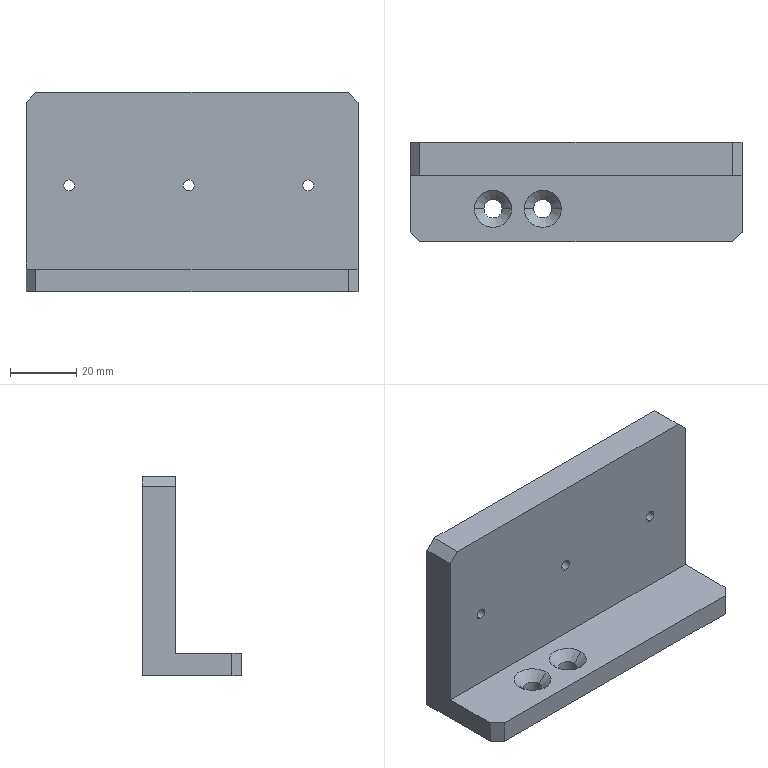Part | SolidWorks | features HoleWzd 2, Chamfer 1, Extrusion 1, ICE 1 | 1 solid | 26 faces | box 100 x 30 x 60 mm | volume 72680 mm3 | plane 12 | cylinder 10 | cone 4 | commonest cylinder face diameters 3.3 x6 5.5 x4
STEP:
#1=CARTESIAN_POINT('',(-12.75,-10.,-26.05));
#2=VERTEX_POINT('',#1);
#3=CARTESIAN_POINT('',(-7.25,-10.,-26.05));
#4=VERTEX_POINT('',#3);
#5=CARTESIAN_POINT('',(-10.,-10.,-26.05));
#6=DIRECTION('',(0.,0.,1.));
#7=DIRECTION('',(1.,0.,0.));
#8=AXIS2_PLACEMENT_3D('',#5,#6,#7);
#9=CIRCLE('',#8,2.75);
#10=EDGE_CURVE('',#2,#4,#9,.T.);
#11=ORIENTED_EDGE('',*,*,#10,.F.);
#12=CARTESIAN_POINT('',(-15.6,-10.,-23.2));
#13=VERTEX_POINT('',#12);
#14=CARTESIAN_POINT('',(-15.6,-10.,-23.2));
#15=DIRECTION('',(-0.7071,0.,0.7071));
#16=VECTOR('',#15,1000.);
#17=LINE('',#14,#16);
#18=EDGE_CURVE('',#2,#13,#17,.T.);
#19=ORIENTED_EDGE('',*,*,#18,.T.);
#20=CARTESIAN_POINT('',(-4.4,-10.,-23.2));
#21=VERTEX_POINT('',#20);
#22=CARTESIAN_POINT('',(-10.,-10.,-23.2));
#23=DIRECTION('',(0.,0.,1.));
#24=DIRECTION('',(1.,0.,0.));
#25=AXIS2_PLACEMENT_3D('',#22,#23,#24);
#26=CIRCLE('',#25,5.6);
#27=EDGE_CURVE('',#13,#21,#26,.T.);
#28=ORIENTED_EDGE('',*,*,#27,.T.);
#29=CARTESIAN_POINT('',(-4.4,-10.,-23.2));
#30=DIRECTION('',(0.7071,0.,0.7071));
#31=VECTOR('',#30,1000.);
#32=LINE('',#29,#31);
#33=EDGE_CURVE('',#4,#21,#32,.T.);
#34=ORIENTED_EDGE('',*,*,#33,.F.);
#35=EDGE_LOOP('',(#11,#19,#28,#34));
#36=FACE_OUTER_BOUND('',#35,.T.);
#37=CARTESIAN_POINT('',(-10.,-10.,-23.2));
#38=DIRECTION('',(0.,0.,1.));
#39=DIRECTION('',(1.,0.,0.));
#40=AXIS2_PLACEMENT_3D('',#37,#38,#39);
#41=CONICAL_SURFACE('',#40,5.6,0.7854);
#42=ADVANCED_FACE('',(#36),#41,.F.);
#43=CARTESIAN_POINT('',(-12.75,-10.,-30.));
#44=VERTEX_POINT('',#43);
#45=CARTESIAN_POINT('',(-7.25,-10.,-30.));
#46=VERTEX_POINT('',#45);
#47=CARTESIAN_POINT('',(-10.,-10.,-30.));
#48=DIRECTION('',(0.,0.,1.));
#49=DIRECTION('',(1.,0.,0.));
#50=AXIS2_PLACEMENT_3D('',#47,#48,#49);
#51=CIRCLE('',#50,2.75);
#52=EDGE_CURVE('',#44,#46,#51,.T.);
#53=ORIENTED_EDGE('',*,*,#52,.F.);
#54=CARTESIAN_POINT('',(-12.75,-10.,-23.2));
#55=DIRECTION('',(0.,0.,1.));
#56=VECTOR('',#55,1000.);
#57=LINE('',#54,#56);
#58=EDGE_CURVE('',#44,#2,#57,.T.);
#59=ORIENTED_EDGE('',*,*,#58,.T.);
#60=ORIENTED_EDGE('',*,*,#10,.T.);
#61=CARTESIAN_POINT('',(-7.25,-10.,-23.2));
#62=DIRECTION('',(0.,0.,1.));
#63=VECTOR('',#62,1000.);
#64=LINE('',#61,#63);
#65=EDGE_CURVE('',#46,#4,#64,.T.);
#66=ORIENTED_EDGE('',*,*,#65,.F.);
#67=EDGE_LOOP('',(#53,#59,#60,#66));
#68=FACE_OUTER_BOUND('',#67,.T.);
#69=CARTESIAN_POINT('',(-10.,-10.,-23.2));
#70=DIRECTION('',(0.,0.,1.));
#71=DIRECTION('',(1.,0.,0.));
#72=AXIS2_PLACEMENT_3D('',#69,#70,#71);
#73=CYLINDRICAL_SURFACE('',#72,2.75);
#74=ADVANCED_FACE('',(#68),#73,.F.);
#75=CARTESIAN_POINT('',(-27.75,-10.,-26.05));
#76=VERTEX_POINT('',#75);
#77=CARTESIAN_POINT('',(-22.25,-10.,-26.05));
#78=VERTEX_POINT('',#77);
#79=CARTESIAN_POINT('',(-25.,-10.,-26.05));
#80=DIRECTION('',(0.,0.,1.));
#81=DIRECTION('',(1.,0.,0.));
#82=AXIS2_PLACEMENT_3D('',#79,#80,#81);
#83=CIRCLE('',#82,2.75);
#84=EDGE_CURVE('',#76,#78,#83,.T.);
#85=ORIENTED_EDGE('',*,*,#84,.F.);
#86=CARTESIAN_POINT('',(-30.6,-10.,-23.2));
#87=VERTEX_POINT('',#86);
#88=CARTESIAN_POINT('',(-30.6,-10.,-23.2));
#89=DIRECTION('',(-0.7071,0.,0.7071));
#90=VECTOR('',#89,1000.);
#91=LINE('',#88,#90);
#92=EDGE_CURVE('',#76,#87,#91,.T.);
#93=ORIENTED_EDGE('',*,*,#92,.T.);
#94=CARTESIAN_POINT('',(-19.4,-10.,-23.2));
#95=VERTEX_POINT('',#94);
#96=CARTESIAN_POINT('',(-25.,-10.,-23.2));
#97=DIRECTION('',(0.,0.,1.));
#98=DIRECTION('',(1.,0.,0.));
#99=AXIS2_PLACEMENT_3D('',#96,#97,#98);
#100=CIRCLE('',#99,5.6);
#101=EDGE_CURVE('',#87,#95,#100,.T.);
#102=ORIENTED_EDGE('',*,*,#101,.T.);
#103=CARTESIAN_POINT('',(-19.4,-10.,-23.2));
#104=DIRECTION('',(0.7071,0.,0.7071));
#105=VECTOR('',#104,1000.);
#106=LINE('',#103,#105);
#107=EDGE_CURVE('',#78,#95,#106,.T.);
#108=ORIENTED_EDGE('',*,*,#107,.F.);
#109=EDGE_LOOP('',(#85,#93,#102,#108));
#110=FACE_OUTER_BOUND('',#109,.T.);
#111=CARTESIAN_POINT('',(-25.,-10.,-23.2));
#112=DIRECTION('',(0.,0.,1.));
#113=DIRECTION('',(1.,0.,0.));
#114=AXIS2_PLACEMENT_3D('',#111,#112,#113);
#115=CONICAL_SURFACE('',#114,5.6,0.7854);
#116=ADVANCED_FACE('',(#110),#115,.F.);
#117=CARTESIAN_POINT('',(-27.75,-10.,-30.));
#118=VERTEX_POINT('',#117);
#119=CARTESIAN_POINT('',(-22.25,-10.,-30.));
#120=VERTEX_POINT('',#119);
#121=CARTESIAN_POINT('',(-25.,-10.,-30.));
#122=DIRECTION('',(0.,0.,1.));
#123=DIRECTION('',(1.,0.,0.));
#124=AXIS2_PLACEMENT_3D('',#121,#122,#123);
#125=CIRCLE('',#124,2.75);
#126=EDGE_CURVE('',#118,#120,#125,.T.);
#127=ORIENTED_EDGE('',*,*,#126,.F.);
#128=CARTESIAN_POINT('',(-27.75,-10.,-23.2));
#129=DIRECTION('',(0.,0.,1.));
#130=VECTOR('',#129,1000.);
#131=LINE('',#128,#130);
#132=EDGE_CURVE('',#118,#76,#131,.T.);
#133=ORIENTED_EDGE('',*,*,#132,.T.);
#134=ORIENTED_EDGE('',*,*,#84,.T.);
#135=CARTESIAN_POINT('',(-22.25,-10.,-23.2));
#136=DIRECTION('',(0.,0.,1.));
#137=VECTOR('',#136,1000.);
#138=LINE('',#135,#137);
#139=EDGE_CURVE('',#120,#78,#138,.T.);
#140=ORIENTED_EDGE('',*,*,#139,.F.);
#141=EDGE_LOOP('',(#127,#133,#134,#140));
#142=FACE_OUTER_BOUND('',#141,.T.);
#143=CARTESIAN_POINT('',(-25.,-10.,-23.2));
#144=DIRECTION('',(0.,0.,1.));
#145=DIRECTION('',(1.,0.,0.));
#146=AXIS2_PLACEMENT_3D('',#143,#144,#145);
#147=CYLINDRICAL_SURFACE('',#146,2.75);
#148=ADVANCED_FACE('',(#142),#147,.F.);
#149=CARTESIAN_POINT('',(35.,0.,0.35));
#150=VERTEX_POINT('',#149);
#151=CARTESIAN_POINT('',(35.,0.,3.65));
#152=VERTEX_POINT('',#151);
#153=CARTESIAN_POINT('',(35.,0.,2.));
#154=DIRECTION('',(0.,1.,0.));
#155=DIRECTION('',(0.,0.,1.));
#156=AXIS2_PLACEMENT_3D('',#153,#154,#155);
#157=CIRCLE('',#156,1.65);
#158=EDGE_CURVE('',#150,#152,#157,.T.);
#159=ORIENTED_EDGE('',*,*,#158,.F.);
#160=CARTESIAN_POINT('',(35.,10.,0.35));
#161=VERTEX_POINT('',#160);
#162=CARTESIAN_POINT('',(35.,10.,0.35));
#163=DIRECTION('',(0.,1.,0.));
#164=VECTOR('',#163,1000.);
#165=LINE('',#162,#164);
#166=EDGE_CURVE('',#150,#161,#165,.T.);
#167=ORIENTED_EDGE('',*,*,#166,.T.);
#168=CARTESIAN_POINT('',(35.,10.,3.65));
#169=VERTEX_POINT('',#168);
#170=CARTESIAN_POINT('',(35.,10.,2.));
#171=DIRECTION('',(0.,1.,0.));
#172=DIRECTION('',(0.,0.,1.));
#173=AXIS2_PLACEMENT_3D('',#170,#171,#172);
#174=CIRCLE('',#173,1.65);
#175=EDGE_CURVE('',#161,#169,#174,.T.);
#176=ORIENTED_EDGE('',*,*,#175,.T.);
#177=CARTESIAN_POINT('',(35.,10.,3.65));
#178=DIRECTION('',(0.,1.,0.));
#179=VECTOR('',#178,1000.);
#180=LINE('',#177,#179);
#181=EDGE_CURVE('',#152,#169,#180,.T.);
#182=ORIENTED_EDGE('',*,*,#181,.F.);
#183=EDGE_LOOP('',(#159,#167,#176,#182));
#184=FACE_OUTER_BOUND('',#183,.T.);
#185=CARTESIAN_POINT('',(35.,10.,2.));
#186=DIRECTION('',(0.,1.,0.));
#187=DIRECTION('',(0.,0.,1.));
#188=AXIS2_PLACEMENT_3D('',#185,#186,#187);
#189=CYLINDRICAL_SURFACE('',#188,1.65);
#190=ADVANCED_FACE('',(#184),#189,.F.);
#191=CARTESIAN_POINT('',(-37.,0.,0.35));
#192=VERTEX_POINT('',#191);
#193=CARTESIAN_POINT('',(-37.,0.,3.65));
#194=VERTEX_POINT('',#193);
#195=CARTESIAN_POINT('',(-37.,0.,2.));
#196=DIRECTION('',(0.,1.,0.));
#197=DIRECTION('',(0.,0.,1.));
#198=AXIS2_PLACEMENT_3D('',#195,#196,#197);
#199=CIRCLE('',#198,1.65);
#200=EDGE_CURVE('',#192,#194,#199,.T.);
#201=ORIENTED_EDGE('',*,*,#200,.F.);
#202=CARTESIAN_POINT('',(-37.,10.,0.35));
#203=VERTEX_POINT('',#202);
#204=CARTESIAN_POINT('',(-37.,10.,0.35));
#205=DIRECTION('',(0.,1.,0.));
#206=VECTOR('',#205,1000.);
#207=LINE('',#204,#206);
#208=EDGE_CURVE('',#192,#203,#207,.T.);
#209=ORIENTED_EDGE('',*,*,#208,.T.);
#210=CARTESIAN_POINT('',(-37.,10.,3.65));
#211=VERTEX_POINT('',#210);
#212=CARTESIAN_POINT('',(-37.,10.,2.));
#213=DIRECTION('',(0.,1.,0.));
#214=DIRECTION('',(0.,0.,1.));
#215=AXIS2_PLACEMENT_3D('',#212,#213,#214);
#216=CIRCLE('',#215,1.65);
#217=EDGE_CURVE('',#203,#211,#216,.T.);
#218=ORIENTED_EDGE('',*,*,#217,.T.);
#219=CARTESIAN_POINT('',(-37.,10.,3.65));
#220=DIRECTION('',(0.,1.,0.));
#221=VECTOR('',#220,1000.);
#222=LINE('',#219,#221);
#223=EDGE_CURVE('',#194,#211,#222,.T.);
#224=ORIENTED_EDGE('',*,*,#223,.F.);
#225=EDGE_LOOP('',(#201,#209,#218,#224));
#226=FACE_OUTER_BOUND('',#225,.T.);
#227=CARTESIAN_POINT('',(-37.,10.,2.));
#228=DIRECTION('',(0.,1.,0.));
#229=DIRECTION('',(0.,0.,1.));
#230=AXIS2_PLACEMENT_3D('',#227,#228,#229);
#231=CYLINDRICAL_SURFACE('',#230,1.65);
#232=ADVANCED_FACE('',(#226),#231,.F.);
#233=CARTESIAN_POINT('',(-1.,0.,0.35));
#234=VERTEX_POINT('',#233);
#235=CARTESIAN_POINT('',(-1.,0.,3.65));
#236=VERTEX_POINT('',#235);
#237=CARTESIAN_POINT('',(-1.,0.,2.));
#238=DIRECTION('',(0.,1.,0.));
#239=DIRECTION('',(0.,0.,1.));
#240=AXIS2_PLACEMENT_3D('',#237,#238,#239);
#241=CIRCLE('',#240,1.65);
#242=EDGE_CURVE('',#234,#236,#241,.T.);
#243=ORIENTED_EDGE('',*,*,#242,.F.);
#244=CARTESIAN_POINT('',(-1.,10.,0.35));
#245=VERTEX_POINT('',#244);
#246=CARTESIAN_POINT('',(-1.,10.,0.35));
#247=DIRECTION('',(0.,1.,0.));
#248=VECTOR('',#247,1000.);
#249=LINE('',#246,#248);
#250=EDGE_CURVE('',#234,#245,#249,.T.);
#251=ORIENTED_EDGE('',*,*,#250,.T.);
#252=CARTESIAN_POINT('',(-1.,10.,3.65));
#253=VERTEX_POINT('',#252);
#254=CARTESIAN_POINT('',(-1.,10.,2.));
#255=DIRECTION('',(0.,1.,0.));
#256=DIRECTION('',(0.,0.,1.));
#257=AXIS2_PLACEMENT_3D('',#254,#255,#256);
#258=CIRCLE('',#257,1.65);
#259=EDGE_CURVE('',#245,#253,#258,.T.);
#260=ORIENTED_EDGE('',*,*,#259,.T.);
#261=CARTESIAN_POINT('',(-1.,10.,3.65));
#262=DIRECTION('',(0.,1.,0.));
#263=VECTOR('',#262,1000.);
#264=LINE('',#261,#263);
#265=EDGE_CURVE('',#236,#253,#264,.T.);
#266=ORIENTED_EDGE('',*,*,#265,.F.);
#267=EDGE_LOOP('',(#243,#251,#260,#266));
#268=FACE_OUTER_BOUND('',#267,.T.);
#269=CARTESIAN_POINT('',(-1.,10.,2.));
#270=DIRECTION('',(0.,1.,0.));
#271=DIRECTION('',(0.,0.,1.));
#272=AXIS2_PLACEMENT_3D('',#269,#270,#271);
#273=CYLINDRICAL_SURFACE('',#272,1.65);
#274=ADVANCED_FACE('',(#268),#273,.F.);
#275=CARTESIAN_POINT('',(35.,0.,2.));
#276=DIRECTION('',(0.,1.,0.));
#277=DIRECTION('',(0.,0.,1.));
#278=AXIS2_PLACEMENT_3D('',#275,#276,#277);
#279=CIRCLE('',#278,1.65);
#280=EDGE_CURVE('',#152,#150,#279,.T.);
#281=ORIENTED_EDGE('',*,*,#280,.T.);
#282=ORIENTED_EDGE('',*,*,#158,.T.);
#283=EDGE_LOOP('',(#281,#282));
#284=FACE_BOUND('',#283,.T.);
#285=CARTESIAN_POINT('',(-37.,0.,2.));
#286=DIRECTION('',(0.,1.,0.));
#287=DIRECTION('',(0.,0.,1.));
#288=AXIS2_PLACEMENT_3D('',#285,#286,#287);
#289=CIRCLE('',#288,1.65);
#290=EDGE_CURVE('',#194,#192,#289,.T.);
#291=ORIENTED_EDGE('',*,*,#290,.T.);
#292=ORIENTED_EDGE('',*,*,#200,.T.);
#293=EDGE_LOOP('',(#291,#292));
#294=FACE_BOUND('',#293,.T.);
#295=CARTESIAN_POINT('',(-1.,0.,2.));
#296=DIRECTION('',(0.,1.,0.));
#297=DIRECTION('',(0.,0.,1.));
#298=AXIS2_PLACEMENT_3D('',#295,#296,#297);
#299=CIRCLE('',#298,1.65);
#300=EDGE_CURVE('',#236,#234,#299,.T.);
#301=ORIENTED_EDGE('',*,*,#300,.T.);
#302=ORIENTED_EDGE('',*,*,#242,.T.);
#303=EDGE_LOOP('',(#301,#302));
#304=FACE_BOUND('',#303,.T.);
#305=CARTESIAN_POINT('',(-47.,0.,30.));
#306=VERTEX_POINT('',#305);
#307=CARTESIAN_POINT('',(47.,0.,30.));
#308=VERTEX_POINT('',#307);
#309=CARTESIAN_POINT('',(-50.,0.,30.));
#310=DIRECTION('',(1.,0.,0.));
#311=VECTOR('',#310,1000.);
#312=LINE('',#309,#311);
#313=EDGE_CURVE('',#306,#308,#312,.T.);
#314=ORIENTED_EDGE('',*,*,#313,.F.);
#315=CARTESIAN_POINT('',(-50.,0.,27.));
#316=VERTEX_POINT('',#315);
#317=CARTESIAN_POINT('',(-47.,0.,30.));
#318=DIRECTION('',(-0.7071,0.,-0.7071));
#319=VECTOR('',#318,1000.);
#320=LINE('',#317,#319);
#321=EDGE_CURVE('',#306,#316,#320,.T.);
#322=ORIENTED_EDGE('',*,*,#321,.T.);
#323=CARTESIAN_POINT('',(-50.,0.,-23.2));
#324=VERTEX_POINT('',#323);
#325=CARTESIAN_POINT('',(-50.,0.,-30.));
#326=DIRECTION('',(0.,0.,1.));
#327=VECTOR('',#326,1000.);
#328=LINE('',#325,#327);
#329=EDGE_CURVE('',#324,#316,#328,.T.);
#330=ORIENTED_EDGE('',*,*,#329,.F.);
#331=CARTESIAN_POINT('',(50.,0.,-23.2));
#332=VERTEX_POINT('',#331);
#333=CARTESIAN_POINT('',(50.,0.,-23.2));
#334=DIRECTION('',(-1.,0.,0.));
#335=VECTOR('',#334,1000.);
#336=LINE('',#333,#335);
#337=EDGE_CURVE('',#332,#324,#336,.T.);
#338=ORIENTED_EDGE('',*,*,#337,.F.);
#339=CARTESIAN_POINT('',(50.,0.,27.));
#340=VERTEX_POINT('',#339);
#341=CARTESIAN_POINT('',(50.,0.,-30.));
#342=DIRECTION('',(0.,0.,-1.));
#343=VECTOR('',#342,1000.);
#344=LINE('',#341,#343);
#345=EDGE_CURVE('',#340,#332,#344,.T.);
#346=ORIENTED_EDGE('',*,*,#345,.F.);
#347=CARTESIAN_POINT('',(50.,0.,27.));
#348=DIRECTION('',(-0.7071,0.,0.7071));
#349=VECTOR('',#348,1000.);
#350=LINE('',#347,#349);
#351=EDGE_CURVE('',#340,#308,#350,.T.);
#352=ORIENTED_EDGE('',*,*,#351,.T.);
#353=EDGE_LOOP('',(#314,#322,#330,#338,#346,#352));
#354=FACE_OUTER_BOUND('',#353,.T.);
#355=CARTESIAN_POINT('',(0.,0.,0.));
#356=DIRECTION('',(0.,1.,0.));
#357=DIRECTION('',(0.,0.,1.));
#358=AXIS2_PLACEMENT_3D('',#355,#356,#357);
#359=PLANE('',#358);
#360=ADVANCED_FACE('',(#284,#294,#304,#354),#359,.F.);
#361=CARTESIAN_POINT('',(50.,10.,27.));
#362=VERTEX_POINT('',#361);
#363=CARTESIAN_POINT('',(50.,10.,-30.));
#364=VERTEX_POINT('',#363);
#365=CARTESIAN_POINT('',(50.,10.,-30.));
#366=DIRECTION('',(0.,0.,-1.));
#367=VECTOR('',#366,1000.);
#368=LINE('',#365,#367);
#369=EDGE_CURVE('',#362,#364,#368,.T.);
#370=ORIENTED_EDGE('',*,*,#369,.F.);
#371=CARTESIAN_POINT('',(50.,10.,27.));
#372=DIRECTION('',(0.,-1.,0.));
#373=VECTOR('',#372,1000.);
#374=LINE('',#371,#373);
#375=EDGE_CURVE('',#362,#340,#374,.T.);
#376=ORIENTED_EDGE('',*,*,#375,.T.);
#377=ORIENTED_EDGE('',*,*,#345,.T.);
#378=CARTESIAN_POINT('',(50.,-17.,-23.2));
#379=VERTEX_POINT('',#378);
#380=CARTESIAN_POINT('',(50.,-20.,-23.2));
#381=DIRECTION('',(0.,1.,0.));
#382=VECTOR('',#381,1000.);
#383=LINE('',#380,#382);
#384=EDGE_CURVE('',#379,#332,#383,.T.);
#385=ORIENTED_EDGE('',*,*,#384,.F.);
#386=CARTESIAN_POINT('',(50.,-17.,-30.));
#387=VERTEX_POINT('',#386);
#388=CARTESIAN_POINT('',(50.,-17.,-30.));
#389=DIRECTION('',(0.,0.,-1.));
#390=VECTOR('',#389,1000.);
#391=LINE('',#388,#390);
#392=EDGE_CURVE('',#379,#387,#391,.T.);
#393=ORIENTED_EDGE('',*,*,#392,.T.);
#394=CARTESIAN_POINT('',(50.,10.,-30.));
#395=DIRECTION('',(0.,-1.,0.));
#396=VECTOR('',#395,1000.);
#397=LINE('',#394,#396);
#398=EDGE_CURVE('',#364,#387,#397,.T.);
#399=ORIENTED_EDGE('',*,*,#398,.F.);
#400=EDGE_LOOP('',(#370,#376,#377,#385,#393,#399));
#401=FACE_OUTER_BOUND('',#400,.T.);
#402=CARTESIAN_POINT('',(50.,10.,-30.));
#403=DIRECTION('',(-1.,0.,0.));
#404=DIRECTION('',(0.,0.,1.));
#405=AXIS2_PLACEMENT_3D('',#402,#403,#404);
#406=PLANE('',#405);
#407=ADVANCED_FACE('',(#401),#406,.F.);
#408=CARTESIAN_POINT('',(-10.,-10.,-30.));
#409=DIRECTION('',(0.,0.,1.));
#410=DIRECTION('',(1.,0.,0.));
#411=AXIS2_PLACEMENT_3D('',#408,#409,#410);
#412=CIRCLE('',#411,2.75);
#413=EDGE_CURVE('',#46,#44,#412,.T.);
#414=ORIENTED_EDGE('',*,*,#413,.T.);
#415=ORIENTED_EDGE('',*,*,#52,.T.);
#416=EDGE_LOOP('',(#414,#415));
#417=FACE_BOUND('',#416,.T.);
#418=CARTESIAN_POINT('',(-25.,-10.,-30.));
#419=DIRECTION('',(0.,0.,1.));
#420=DIRECTION('',(1.,0.,0.));
#421=AXIS2_PLACEMENT_3D('',#418,#419,#420);
#422=CIRCLE('',#421,2.75);
#423=EDGE_CURVE('',#120,#118,#422,.T.);
#424=ORIENTED_EDGE('',*,*,#423,.T.);
#425=ORIENTED_EDGE('',*,*,#126,.T.);
#426=EDGE_LOOP('',(#424,#425));
#427=FACE_BOUND('',#426,.T.);
#428=CARTESIAN_POINT('',(-47.,-20.,-30.));
#429=VERTEX_POINT('',#428);
#430=CARTESIAN_POINT('',(47.,-20.,-30.));
#431=VERTEX_POINT('',#430);
#432=CARTESIAN_POINT('',(50.,-20.,-30.));
#433=DIRECTION('',(1.,0.,0.));
#434=VECTOR('',#433,1000.);
#435=LINE('',#432,#434);
#436=EDGE_CURVE('',#429,#431,#435,.T.);
#437=ORIENTED_EDGE('',*,*,#436,.F.);
#438=CARTESIAN_POINT('',(-50.,-17.,-30.));
#439=VERTEX_POINT('',#438);
#440=CARTESIAN_POINT('',(-47.,-20.,-30.));
#441=DIRECTION('',(-0.7071,0.7071,0.));
#442=VECTOR('',#441,1000.);
#443=LINE('',#440,#442);
#444=EDGE_CURVE('',#429,#439,#443,.T.);
#445=ORIENTED_EDGE('',*,*,#444,.T.);
#446=CARTESIAN_POINT('',(-50.,10.,-30.));
#447=VERTEX_POINT('',#446);
#448=CARTESIAN_POINT('',(-50.,10.,-30.));
#449=DIRECTION('',(0.,-1.,0.));
#450=VECTOR('',#449,1000.);
#451=LINE('',#448,#450);
#452=EDGE_CURVE('',#447,#439,#451,.T.);
#453=ORIENTED_EDGE('',*,*,#452,.F.);
#454=CARTESIAN_POINT('',(-50.,10.,-30.));
#455=DIRECTION('',(-1.,0.,0.));
#456=VECTOR('',#455,1000.);
#457=LINE('',#454,#456);
#458=EDGE_CURVE('',#364,#447,#457,.T.);
#459=ORIENTED_EDGE('',*,*,#458,.F.);
#460=ORIENTED_EDGE('',*,*,#398,.T.);
#461=CARTESIAN_POINT('',(47.,-20.,-30.));
#462=DIRECTION('',(-0.7071,-0.7071,0.));
#463=VECTOR('',#462,1000.);
#464=LINE('',#461,#463);
#465=EDGE_CURVE('',#387,#431,#464,.T.);
#466=ORIENTED_EDGE('',*,*,#465,.T.);
#467=EDGE_LOOP('',(#437,#445,#453,#459,#460,#466));
#468=FACE_OUTER_BOUND('',#467,.T.);
#469=CARTESIAN_POINT('',(-50.,10.,-30.));
#470=DIRECTION('',(0.,0.,1.));
#471=DIRECTION('',(1.,0.,0.));
#472=AXIS2_PLACEMENT_3D('',#469,#470,#471);
#473=PLANE('',#472);
#474=ADVANCED_FACE('',(#417,#427,#468),#473,.F.);
#475=ORIENTED_EDGE('',*,*,#452,.T.);
#476=CARTESIAN_POINT('',(-50.,-17.,-23.2));
#477=VERTEX_POINT('',#476);
#478=CARTESIAN_POINT('',(-50.,-17.,-23.2));
#479=DIRECTION('',(0.,0.,1.));
#480=VECTOR('',#479,1000.);
#481=LINE('',#478,#480);
#482=EDGE_CURVE('',#439,#477,#481,.T.);
#483=ORIENTED_EDGE('',*,*,#482,.T.);
#484=CARTESIAN_POINT('',(-50.,-20.,-23.2));
#485=DIRECTION('',(0.,1.,0.));
#486=VECTOR('',#485,1000.);
#487=LINE('',#484,#486);
#488=EDGE_CURVE('',#477,#324,#487,.T.);
#489=ORIENTED_EDGE('',*,*,#488,.T.);
#490=ORIENTED_EDGE('',*,*,#329,.T.);
#491=CARTESIAN_POINT('',(-50.,10.,27.));
#492=VERTEX_POINT('',#491);
#493=CARTESIAN_POINT('',(-50.,10.,27.));
#494=DIRECTION('',(0.,1.,0.));
#495=VECTOR('',#494,1000.);
#496=LINE('',#493,#495);
#497=EDGE_CURVE('',#316,#492,#496,.T.);
#498=ORIENTED_EDGE('',*,*,#497,.T.);
#499=CARTESIAN_POINT('',(-50.,10.,-30.));
#500=DIRECTION('',(0.,0.,1.));
#501=VECTOR('',#500,1000.);
#502=LINE('',#499,#501);
#503=EDGE_CURVE('',#447,#492,#502,.T.);
#504=ORIENTED_EDGE('',*,*,#503,.F.);
#505=EDGE_LOOP('',(#475,#483,#489,#490,#498,#504));
#506=FACE_OUTER_BOUND('',#505,.T.);
#507=CARTESIAN_POINT('',(-50.,10.,-30.));
#508=DIRECTION('',(1.,0.,0.));
#509=DIRECTION('',(0.,0.,-1.));
#510=AXIS2_PLACEMENT_3D('',#507,#508,#509);
#511=PLANE('',#510);
#512=ADVANCED_FACE('',(#506),#511,.F.);
#513=CARTESIAN_POINT('',(-47.,10.,30.));
#514=VERTEX_POINT('',#513);
#515=CARTESIAN_POINT('',(47.,10.,30.));
#516=VERTEX_POINT('',#515);
#517=CARTESIAN_POINT('',(-50.,10.,30.));
#518=DIRECTION('',(1.,0.,0.));
#519=VECTOR('',#518,1000.);
#520=LINE('',#517,#519);
#521=EDGE_CURVE('',#514,#516,#520,.T.);
#522=ORIENTED_EDGE('',*,*,#521,.F.);
#523=CARTESIAN_POINT('',(-47.,10.,30.));
#524=DIRECTION('',(0.,-1.,0.));
#525=VECTOR('',#524,1000.);
#526=LINE('',#523,#525);
#527=EDGE_CURVE('',#514,#306,#526,.T.);
#528=ORIENTED_EDGE('',*,*,#527,.T.);
#529=ORIENTED_EDGE('',*,*,#313,.T.);
#530=CARTESIAN_POINT('',(47.,10.,30.));
#531=DIRECTION('',(0.,1.,0.));
#532=VECTOR('',#531,1000.);
#533=LINE('',#530,#532);
#534=EDGE_CURVE('',#308,#516,#533,.T.);
#535=ORIENTED_EDGE('',*,*,#534,.T.);
#536=EDGE_LOOP('',(#522,#528,#529,#535));
#537=FACE_OUTER_BOUND('',#536,.T.);
#538=CARTESIAN_POINT('',(-50.,10.,30.));
#539=DIRECTION('',(0.,0.,-1.));
#540=DIRECTION('',(-1.,0.,0.));
#541=AXIS2_PLACEMENT_3D('',#538,#539,#540);
#542=PLANE('',#541);
#543=ADVANCED_FACE('',(#537),#542,.F.);
#544=CARTESIAN_POINT('',(35.,10.,2.));
#545=DIRECTION('',(0.,1.,0.));
#546=DIRECTION('',(0.,0.,1.));
#547=AXIS2_PLACEMENT_3D('',#544,#545,#546);
#548=CIRCLE('',#547,1.65);
#549=EDGE_CURVE('',#169,#161,#548,.T.);
#550=ORIENTED_EDGE('',*,*,#549,.F.);
#551=ORIENTED_EDGE('',*,*,#175,.F.);
#552=EDGE_LOOP('',(#550,#551));
#553=FACE_BOUND('',#552,.T.);
#554=CARTESIAN_POINT('',(-37.,10.,2.));
#555=DIRECTION('',(0.,1.,0.));
#556=DIRECTION('',(0.,0.,1.));
#557=AXIS2_PLACEMENT_3D('',#554,#555,#556);
#558=CIRCLE('',#557,1.65);
#559=EDGE_CURVE('',#211,#203,#558,.T.);
#560=ORIENTED_EDGE('',*,*,#559,.F.);
#561=ORIENTED_EDGE('',*,*,#217,.F.);
#562=EDGE_LOOP('',(#560,#561));
#563=FACE_BOUND('',#562,.T.);
#564=CARTESIAN_POINT('',(-1.,10.,2.));
#565=DIRECTION('',(0.,1.,0.));
#566=DIRECTION('',(0.,0.,1.));
#567=AXIS2_PLACEMENT_3D('',#564,#565,#566);
#568=CIRCLE('',#567,1.65);
#569=EDGE_CURVE('',#253,#245,#568,.T.);
#570=ORIENTED_EDGE('',*,*,#569,.F.);
#571=ORIENTED_EDGE('',*,*,#259,.F.);
#572=EDGE_LOOP('',(#570,#571));
#573=FACE_BOUND('',#572,.T.);
#574=ORIENTED_EDGE('',*,*,#503,.T.);
#575=CARTESIAN_POINT('',(-38.5,10.,38.5));
#576=DIRECTION('',(0.7071,0.,0.7071));
#577=VECTOR('',#576,1000.);
#578=LINE('',#575,#577);
#579=EDGE_CURVE('',#492,#514,#578,.T.);
#580=ORIENTED_EDGE('',*,*,#579,.T.);
#581=ORIENTED_EDGE('',*,*,#521,.T.);
#582=CARTESIAN_POINT('',(38.5,10.,38.5));
#583=DIRECTION('',(0.7071,0.,-0.7071));
#584=VECTOR('',#583,1000.);
#585=LINE('',#582,#584);
#586=EDGE_CURVE('',#516,#362,#585,.T.);
#587=ORIENTED_EDGE('',*,*,#586,.T.);
#588=ORIENTED_EDGE('',*,*,#369,.T.);
#589=ORIENTED_EDGE('',*,*,#458,.T.);
#590=EDGE_LOOP('',(#574,#580,#581,#587,#588,#589));
#591=FACE_OUTER_BOUND('',#590,.T.);
#592=CARTESIAN_POINT('',(0.,10.,0.));
#593=DIRECTION('',(0.,1.,0.));
#594=DIRECTION('',(0.,0.,1.));
#595=AXIS2_PLACEMENT_3D('',#592,#593,#594);
#596=PLANE('',#595);
#597=ADVANCED_FACE('',(#553,#563,#573,#591),#596,.T.);
#598=CARTESIAN_POINT('',(-10.,-10.,-23.2));
#599=DIRECTION('',(0.,0.,1.));
#600=DIRECTION('',(1.,0.,0.));
#601=AXIS2_PLACEMENT_3D('',#598,#599,#600);
#602=CIRCLE('',#601,5.6);
#603=EDGE_CURVE('',#21,#13,#602,.T.);
#604=ORIENTED_EDGE('',*,*,#603,.F.);
#605=ORIENTED_EDGE('',*,*,#27,.F.);
#606=EDGE_LOOP('',(#604,#605));
#607=FACE_BOUND('',#606,.T.);
#608=CARTESIAN_POINT('',(-25.,-10.,-23.2));
#609=DIRECTION('',(0.,0.,1.));
#610=DIRECTION('',(1.,0.,0.));
#611=AXIS2_PLACEMENT_3D('',#608,#609,#610);
#612=CIRCLE('',#611,5.6);
#613=EDGE_CURVE('',#95,#87,#612,.T.);
#614=ORIENTED_EDGE('',*,*,#613,.F.);
#615=ORIENTED_EDGE('',*,*,#101,.F.);
#616=EDGE_LOOP('',(#614,#615));
#617=FACE_BOUND('',#616,.T.);
#618=ORIENTED_EDGE('',*,*,#488,.F.);
#619=CARTESIAN_POINT('',(-47.,-20.,-23.2));
#620=VERTEX_POINT('',#619);
#621=CARTESIAN_POINT('',(-47.,-20.,-23.2));
#622=DIRECTION('',(0.7071,-0.7071,0.));
#623=VECTOR('',#622,1000.);
#624=LINE('',#621,#623);
#625=EDGE_CURVE('',#477,#620,#624,.T.);
#626=ORIENTED_EDGE('',*,*,#625,.T.);
#627=CARTESIAN_POINT('',(47.,-20.,-23.2));
#628=VERTEX_POINT('',#627);
#629=CARTESIAN_POINT('',(50.,-20.,-23.2));
#630=DIRECTION('',(-1.,0.,0.));
#631=VECTOR('',#630,1000.);
#632=LINE('',#629,#631);
#633=EDGE_CURVE('',#628,#620,#632,.T.);
#634=ORIENTED_EDGE('',*,*,#633,.F.);
#635=CARTESIAN_POINT('',(47.,-20.,-23.2));
#636=DIRECTION('',(0.7071,0.7071,0.));
#637=VECTOR('',#636,1000.);
#638=LINE('',#635,#637);
#639=EDGE_CURVE('',#628,#379,#638,.T.);
#640=ORIENTED_EDGE('',*,*,#639,.T.);
#641=ORIENTED_EDGE('',*,*,#384,.T.);
#642=ORIENTED_EDGE('',*,*,#337,.T.);
#643=EDGE_LOOP('',(#618,#626,#634,#640,#641,#642));
#644=FACE_OUTER_BOUND('',#643,.T.);
#645=CARTESIAN_POINT('',(50.,-20.,-23.2));
#646=DIRECTION('',(0.,0.,-1.));
#647=DIRECTION('',(-1.,0.,0.));
#648=AXIS2_PLACEMENT_3D('',#645,#646,#647);
#649=PLANE('',#648);
#650=ADVANCED_FACE('',(#607,#617,#644),#649,.F.);
#651=ORIENTED_EDGE('',*,*,#633,.T.);
#652=CARTESIAN_POINT('',(-47.,-20.,-30.));
#653=DIRECTION('',(0.,0.,-1.));
#654=VECTOR('',#653,1000.);
#655=LINE('',#652,#654);
#656=EDGE_CURVE('',#620,#429,#655,.T.);
#657=ORIENTED_EDGE('',*,*,#656,.T.);
#658=ORIENTED_EDGE('',*,*,#436,.T.);
#659=CARTESIAN_POINT('',(47.,-20.,-23.2));
#660=DIRECTION('',(0.,0.,1.));
#661=VECTOR('',#660,1000.);
#662=LINE('',#659,#661);
#663=EDGE_CURVE('',#431,#628,#662,.T.);
#664=ORIENTED_EDGE('',*,*,#663,.T.);
#665=EDGE_LOOP('',(#651,#657,#658,#664));
#666=FACE_OUTER_BOUND('',#665,.T.);
#667=CARTESIAN_POINT('',(0.,-20.,0.));
#668=DIRECTION('',(0.,-1.,0.));
#669=DIRECTION('',(0.,0.,-1.));
#670=AXIS2_PLACEMENT_3D('',#667,#668,#669);
#671=PLANE('',#670);
#672=ADVANCED_FACE('',(#666),#671,.T.);
#673=ORIENTED_EDGE('',*,*,#625,.F.);
#674=ORIENTED_EDGE('',*,*,#482,.F.);
#675=ORIENTED_EDGE('',*,*,#444,.F.);
#676=ORIENTED_EDGE('',*,*,#656,.F.);
#677=EDGE_LOOP('',(#673,#674,#675,#676));
#678=FACE_OUTER_BOUND('',#677,.T.);
#679=CARTESIAN_POINT('',(-47.,-20.,0.));
#680=DIRECTION('',(-0.7071,-0.7071,0.));
#681=DIRECTION('',(0.,0.,1.));
#682=AXIS2_PLACEMENT_3D('',#679,#680,#681);
#683=PLANE('',#682);
#684=ADVANCED_FACE('',(#678),#683,.T.);
#685=ORIENTED_EDGE('',*,*,#579,.F.);
#686=ORIENTED_EDGE('',*,*,#497,.F.);
#687=ORIENTED_EDGE('',*,*,#321,.F.);
#688=ORIENTED_EDGE('',*,*,#527,.F.);
#689=EDGE_LOOP('',(#685,#686,#687,#688));
#690=FACE_OUTER_BOUND('',#689,.T.);
#691=CARTESIAN_POINT('',(-47.,10.,30.));
#692=DIRECTION('',(0.7071,0.,-0.7071));
#693=DIRECTION('',(0.,-1.,0.));
#694=AXIS2_PLACEMENT_3D('',#691,#692,#693);
#695=PLANE('',#694);
#696=ADVANCED_FACE('',(#690),#695,.F.);
#697=ORIENTED_EDGE('',*,*,#586,.F.);
#698=ORIENTED_EDGE('',*,*,#534,.F.);
#699=ORIENTED_EDGE('',*,*,#351,.F.);
#700=ORIENTED_EDGE('',*,*,#375,.F.);
#701=EDGE_LOOP('',(#697,#698,#699,#700));
#702=FACE_OUTER_BOUND('',#701,.T.);
#703=CARTESIAN_POINT('',(50.,10.,27.));
#704=DIRECTION('',(-0.7071,0.,-0.7071));
#705=DIRECTION('',(0.,-1.,0.));
#706=AXIS2_PLACEMENT_3D('',#703,#704,#705);
#707=PLANE('',#706);
#708=ADVANCED_FACE('',(#702),#707,.F.);
#709=ORIENTED_EDGE('',*,*,#465,.F.);
#710=ORIENTED_EDGE('',*,*,#392,.F.);
#711=ORIENTED_EDGE('',*,*,#639,.F.);
#712=ORIENTED_EDGE('',*,*,#663,.F.);
#713=EDGE_LOOP('',(#709,#710,#711,#712));
#714=FACE_OUTER_BOUND('',#713,.T.);
#715=CARTESIAN_POINT('',(47.,-20.,0.));
#716=DIRECTION('',(0.7071,-0.7071,0.));
#717=DIRECTION('',(0.,0.,-1.));
#718=AXIS2_PLACEMENT_3D('',#715,#716,#717);
#719=PLANE('',#718);
#720=ADVANCED_FACE('',(#714),#719,.T.);
#721=ORIENTED_EDGE('',*,*,#250,.F.);
#722=ORIENTED_EDGE('',*,*,#300,.F.);
#723=ORIENTED_EDGE('',*,*,#265,.T.);
#724=ORIENTED_EDGE('',*,*,#569,.T.);
#725=EDGE_LOOP('',(#721,#722,#723,#724));
#726=FACE_OUTER_BOUND('',#725,.T.);
#727=CARTESIAN_POINT('',(-1.,10.,2.));
#728=DIRECTION('',(0.,1.,0.));
#729=DIRECTION('',(0.,0.,1.));
#730=AXIS2_PLACEMENT_3D('',#727,#728,#729);
#731=CYLINDRICAL_SURFACE('',#730,1.65);
#732=ADVANCED_FACE('',(#726),#731,.F.);
#733=ORIENTED_EDGE('',*,*,#208,.F.);
#734=ORIENTED_EDGE('',*,*,#290,.F.);
#735=ORIENTED_EDGE('',*,*,#223,.T.);
#736=ORIENTED_EDGE('',*,*,#559,.T.);
#737=EDGE_LOOP('',(#733,#734,#735,#736));
#738=FACE_OUTER_BOUND('',#737,.T.);
#739=CARTESIAN_POINT('',(-37.,10.,2.));
#740=DIRECTION('',(0.,1.,0.));
#741=DIRECTION('',(0.,0.,1.));
#742=AXIS2_PLACEMENT_3D('',#739,#740,#741);
#743=CYLINDRICAL_SURFACE('',#742,1.65);
#744=ADVANCED_FACE('',(#738),#743,.F.);
#745=ORIENTED_EDGE('',*,*,#166,.F.);
#746=ORIENTED_EDGE('',*,*,#280,.F.);
#747=ORIENTED_EDGE('',*,*,#181,.T.);
#748=ORIENTED_EDGE('',*,*,#549,.T.);
#749=EDGE_LOOP('',(#745,#746,#747,#748));
#750=FACE_OUTER_BOUND('',#749,.T.);
#751=CARTESIAN_POINT('',(35.,10.,2.));
#752=DIRECTION('',(0.,1.,0.));
#753=DIRECTION('',(0.,0.,1.));
#754=AXIS2_PLACEMENT_3D('',#751,#752,#753);
#755=CYLINDRICAL_SURFACE('',#754,1.65);
#756=ADVANCED_FACE('',(#750),#755,.F.);
#757=ORIENTED_EDGE('',*,*,#132,.F.);
#758=ORIENTED_EDGE('',*,*,#423,.F.);
#759=ORIENTED_EDGE('',*,*,#139,.T.);
#760=CARTESIAN_POINT('',(-25.,-10.,-26.05));
#761=DIRECTION('',(0.,0.,1.));
#762=DIRECTION('',(1.,0.,0.));
#763=AXIS2_PLACEMENT_3D('',#760,#761,#762);
#764=CIRCLE('',#763,2.75);
#765=EDGE_CURVE('',#78,#76,#764,.T.);
#766=ORIENTED_EDGE('',*,*,#765,.T.);
#767=EDGE_LOOP('',(#757,#758,#759,#766));
#768=FACE_OUTER_BOUND('',#767,.T.);
#769=CARTESIAN_POINT('',(-25.,-10.,-23.2));
#770=DIRECTION('',(0.,0.,1.));
#771=DIRECTION('',(1.,0.,0.));
#772=AXIS2_PLACEMENT_3D('',#769,#770,#771);
#773=CYLINDRICAL_SURFACE('',#772,2.75);
#774=ADVANCED_FACE('',(#768),#773,.F.);
#775=ORIENTED_EDGE('',*,*,#92,.F.);
#776=ORIENTED_EDGE('',*,*,#765,.F.);
#777=ORIENTED_EDGE('',*,*,#107,.T.);
#778=ORIENTED_EDGE('',*,*,#613,.T.);
#779=EDGE_LOOP('',(#775,#776,#777,#778));
#780=FACE_OUTER_BOUND('',#779,.T.);
#781=CARTESIAN_POINT('',(-25.,-10.,-23.2));
#782=DIRECTION('',(0.,0.,1.));
#783=DIRECTION('',(1.,0.,0.));
#784=AXIS2_PLACEMENT_3D('',#781,#782,#783);
#785=CONICAL_SURFACE('',#784,5.6,0.7854);
#786=ADVANCED_FACE('',(#780),#785,.F.);
#787=ORIENTED_EDGE('',*,*,#58,.F.);
#788=ORIENTED_EDGE('',*,*,#413,.F.);
#789=ORIENTED_EDGE('',*,*,#65,.T.);
#790=CARTESIAN_POINT('',(-10.,-10.,-26.05));
#791=DIRECTION('',(0.,0.,1.));
#792=DIRECTION('',(1.,0.,0.));
#793=AXIS2_PLACEMENT_3D('',#790,#791,#792);
#794=CIRCLE('',#793,2.75);
#795=EDGE_CURVE('',#4,#2,#794,.T.);
#796=ORIENTED_EDGE('',*,*,#795,.T.);
#797=EDGE_LOOP('',(#787,#788,#789,#796));
#798=FACE_OUTER_BOUND('',#797,.T.);
#799=CARTESIAN_POINT('',(-10.,-10.,-23.2));
#800=DIRECTION('',(0.,0.,1.));
#801=DIRECTION('',(1.,0.,0.));
#802=AXIS2_PLACEMENT_3D('',#799,#800,#801);
#803=CYLINDRICAL_SURFACE('',#802,2.75);
#804=ADVANCED_FACE('',(#798),#803,.F.);
#805=ORIENTED_EDGE('',*,*,#18,.F.);
#806=ORIENTED_EDGE('',*,*,#795,.F.);
#807=ORIENTED_EDGE('',*,*,#33,.T.);
#808=ORIENTED_EDGE('',*,*,#603,.T.);
#809=EDGE_LOOP('',(#805,#806,#807,#808));
#810=FACE_OUTER_BOUND('',#809,.T.);
#811=CARTESIAN_POINT('',(-10.,-10.,-23.2));
#812=DIRECTION('',(0.,0.,1.));
#813=DIRECTION('',(1.,0.,0.));
#814=AXIS2_PLACEMENT_3D('',#811,#812,#813);
#815=CONICAL_SURFACE('',#814,5.6,0.7854);
#816=ADVANCED_FACE('',(#810),#815,.F.);
#817=CLOSED_SHELL('',(#42,#74,#116,#148,#190,#232,#274,#360,#407,#474,#512,#543,#597,#650,#672,#684,#696,#708,#720,#732,#744,#756,#774,#786,#804,#816));
#818=MANIFOLD_SOLID_BREP('',#817);
#819=CARTESIAN_POINT('',(0.,0.,0.));
#820=DIRECTION('',(0.,0.,1.));
#821=DIRECTION('',(1.,0.,0.));
#822=AXIS2_PLACEMENT_3D('',#819,#820,#821);
#823=(LENGTH_UNIT()NAMED_UNIT(*)SI_UNIT(.MILLI.,.METRE.));
#824=UNCERTAINTY_MEASURE_WITH_UNIT(LENGTH_MEASURE(0.00001),#823,'','');
#825=(NAMED_UNIT(*)PLANE_ANGLE_UNIT()SI_UNIT($,.RADIAN.));
#826=(NAMED_UNIT(*)SI_UNIT($,.STERADIAN.)SOLID_ANGLE_UNIT());
#827=(GEOMETRIC_REPRESENTATION_CONTEXT(3)GLOBAL_UNCERTAINTY_ASSIGNED_CONTEXT((#824))GLOBAL_UNIT_ASSIGNED_CONTEXT((#823,#825,#826))REPRESENTATION_CONTEXT('',''));
#828=ADVANCED_BREP_SHAPE_REPRESENTATION('',(#818,#822),#827);